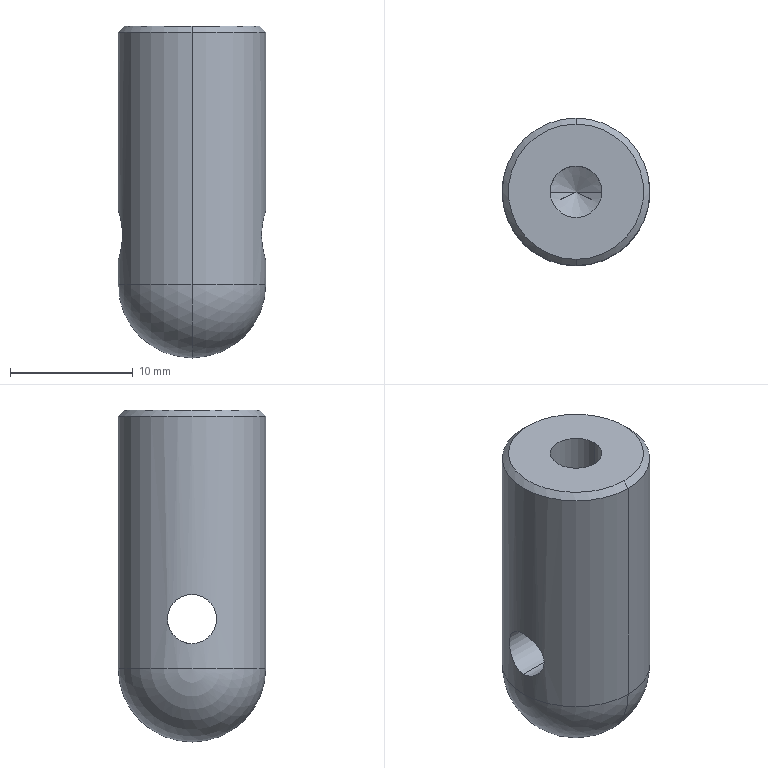Part | STEP file | 227H056251 Pin_Default | 1 solid | 13 faces | box 12 x 12 x 27 mm | volume 2502 mm3 | cylinder 6 | cone 4 | sphere 2 | plane 1 | commonest cylinder face diameters 4 x2 4.2 x2 12 x2